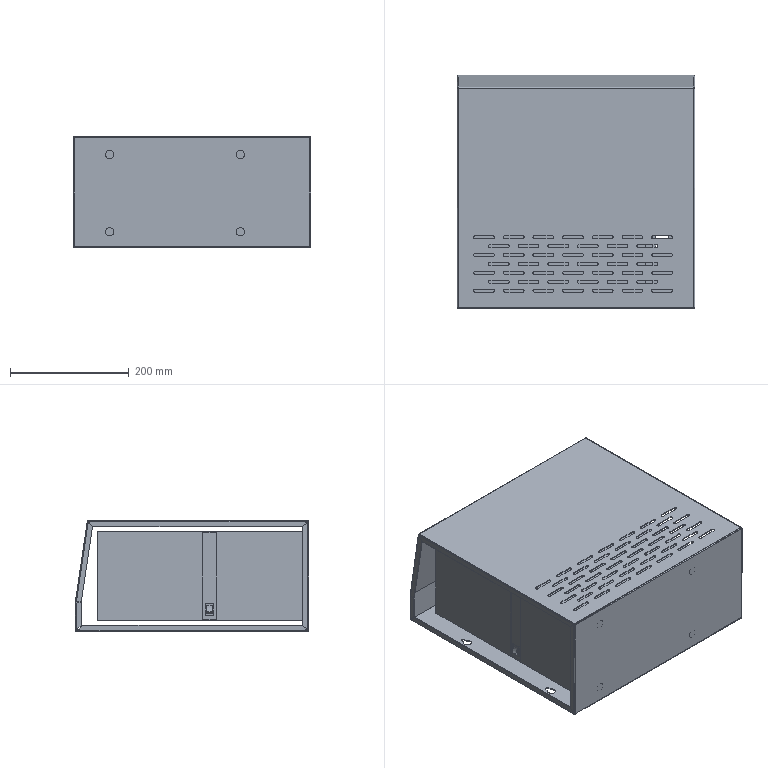Part | SolidWorks | 2 solids | 415 faces | box 400.001 x 393 x 186.5 mm | volume 15923225 mm3 | plane 202 | cylinder 193 | spline 20 | commonest cylinder face diameters 5 x138 0.4 x14 3.4 x14 13 x8 14 x8 22 x6